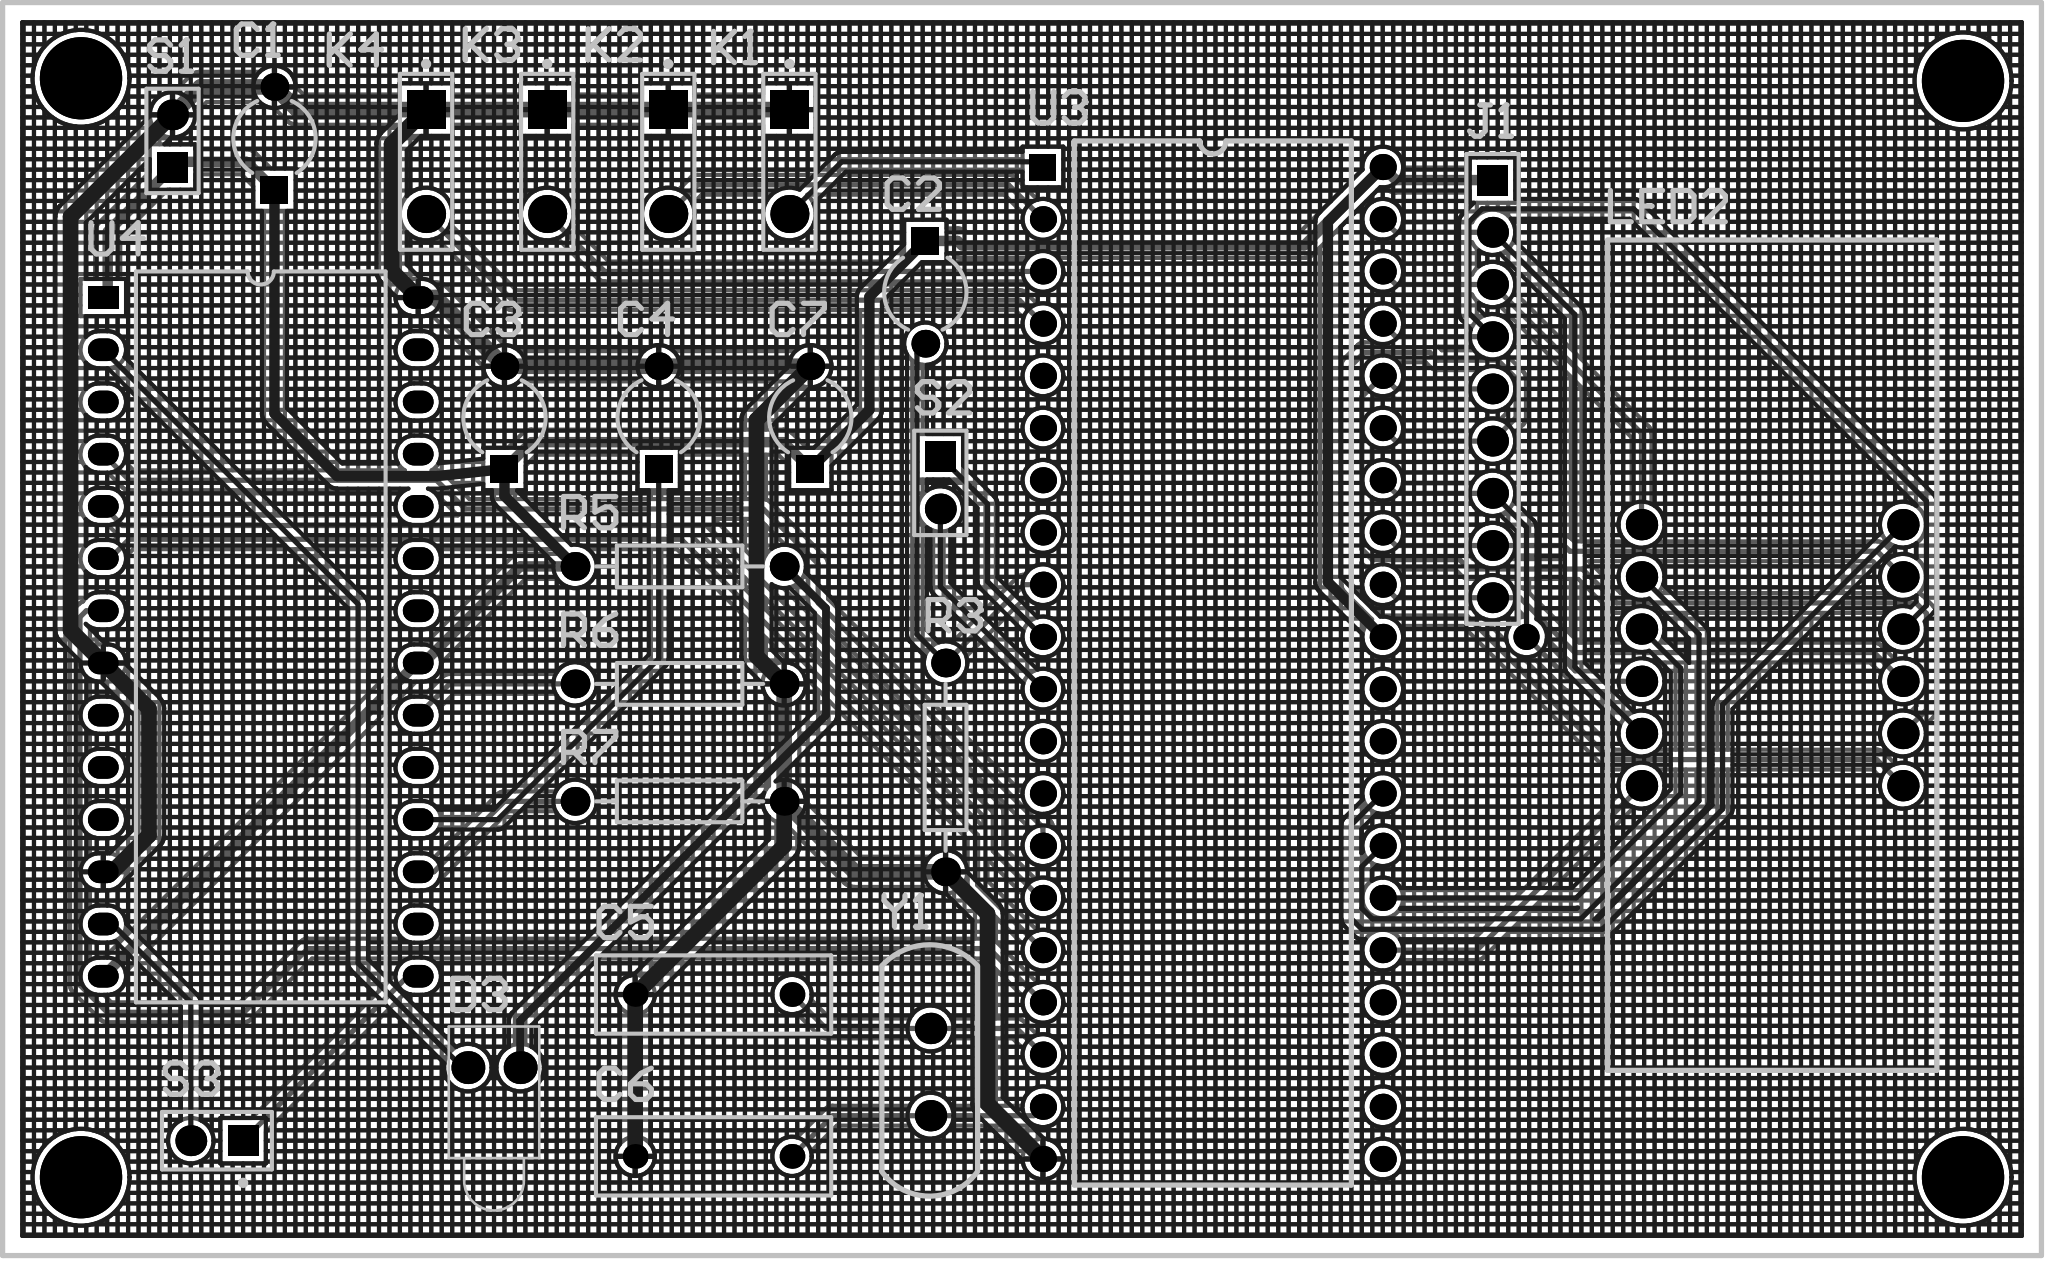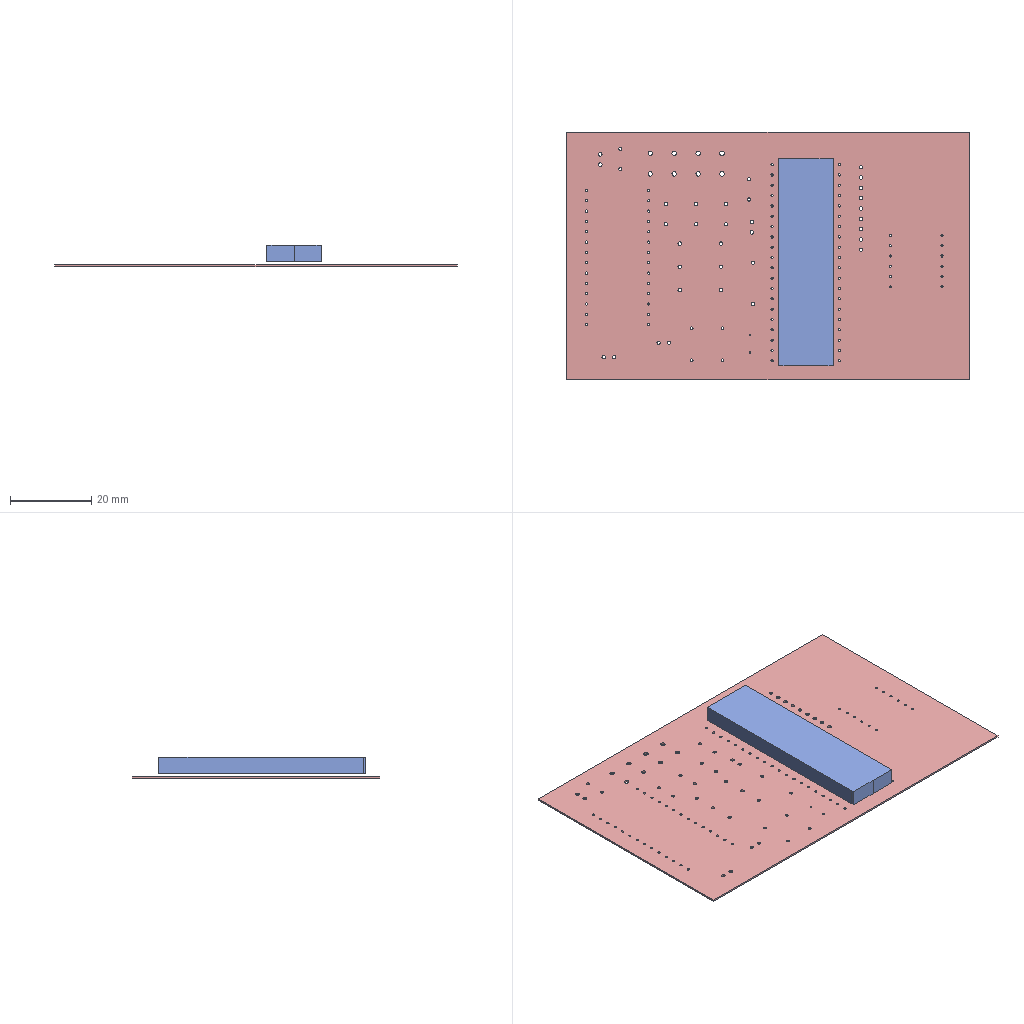Circuit board layout | Altium Designer | box 99.1 x 61 x 5.2 mm
Layer stack:
# Altium Designer layer stack of  (unit mm; dielectric type: 0 none, 1 core, 2 prepreg, 3 surface material)
index,name,kind,layer,copper_thickness_mm,dielectric_type,dielectric_thickness_mm,dielectric_material,dielectric_constant
0,Top Paste,other,,,,,,
1,Top Overlay,other,,,,,,
2,Top Solder,dielectric,,,3,0.0102,Solder Resist,3.5
3,Top Layer,copper,Top Layer,0.0356,,,,
4,Dielectric 1,dielectric,,,0,0.32,FR-4,4.8
5,Bottom Layer,copper,Bottom Layer,0.0356,,,,
6,Bottom Solder,dielectric,,,3,0.0102,Solder Resist,3.5
7,Bottom Overlay,other,,,,,,
8,Bottom Paste,other,,,,,,
# drill layer pairs: low layer,high layer
drill_pair,Top Layer,Bottom Layer
Part placement:
Designator,Comment,Layer,Footprint,Center-X(mm),Center-Y(mm),Rotation
U3,89c51,TopLayer,89c51,104.521,66.929,0
Y1,Component_1,TopLayer,XTAL,90.805,47.026,180
U4,Component_1,TopLayer,ISD1730,58.263,68.199,0
S3,Speaker,TopLayer,PIN2,56.134,43.688,180
S2,Header 2,TopLayer,HDR1X2,91.281,75.692,270
S1,Header 2,TopLayer,HDR1X2,53.975,92.329,90
R7,Res2,TopLayer,AXIAL-0.4,78.613,60.198,180
R6,Res2,TopLayer,AXIAL-0.4,78.613,65.913,180
R5,Res2,TopLayer,AXIAL-0.4,78.613,71.628,360
R3,Res2,TopLayer,AXIAL-0.4,91.535,61.849,90
LED2,Dpy Red-CA,TopLayer,四位数码管,131.699,67.31,90
K4,SW-PB,TopLayer,SPST-2,66.294,91.313,270
K3,SW-PB,TopLayer,SPST-2,72.178,91.313,270
K2,SW-PB,TopLayer,SPST-2,78.063,91.313,270
K1,SW-PB,TopLayer,SPST-2,83.947,91.313,270
J1,Header 9,TopLayer,HDR1X9,118.11,80.264,270
D3,LED1,TopLayer,LED-1,69.596,47.244,270
C7,Cap2,TopLayer,CAPR5-4X5,84.963,78.867,90
C6,Cap,TopLayer,RAD-0.3,80.264,42.926,360
C5,Cap,TopLayer,RAD-0.3,80.264,50.8,360
C4,Cap2,TopLayer,CAPR5-4X5,77.597,78.867,90
C3,Cap2,TopLayer,CAPR5-4X5,70.104,78.867,90
C2,Cap2,TopLayer,CAPR5-4X5,90.551,84.963,270
C1,Cap2,TopLayer,CAPR5-4X5,58.928,92.456,90
Pad and via stacks:
# Altium Designer via and pad stacks of  (unit mm). Each distinct definition once, with the count of objects using it.
# via: kind,start_layer,end_layer,hole_mm,diameter_mm,mode(0 simple;1 top-mid-bottom;2 full stack),diameter_per_layer,count,example_net
# pad: kind,layer,hole_mm,hole_type(0 round;1 square;2 slot),plating,top_size,top_shape(1 round;2 rect;3 octagon;9 rounded rect),mid_size,bottom_size,mode,footprint,size_per_layer,count,example
pad,Multi-Layer,1.1,0,plated,1.85x1.85,2,1.85x1.85,1.85x1.85,0,SPST-2,,4,K1.1
pad,Multi-Layer,1.1,0,plated,1.85x1.85,1,1.85x1.85,1.85x1.85,0,SPST-2,,4,K1.2
pad,Multi-Layer,0.5588,0,plated,1.27x1.27,1,1.27x1.27,1.27x1.27,0,89c51,,39,U3.21
pad,Multi-Layer,0.5588,0,plated,1.27x1.27,2,1.27x1.27,1.27x1.27,0,89c51,,1,U3.1
pad,Multi-Layer,0.51,0,plated,1.524x1.524,1,1.524x1.524,1.524x1.524,0,\u00CB\u00C4\u00CE\u00BB\u00CA\u00FD\u00C2\u00EB\u00B9\u00DC,,12,LED2.1
pad,Multi-Layer,0.9,0,plated,1.5x1.5,2,1.5x1.5,1.5x1.5,0,HDR1X2,,2,S1.1
pad,Multi-Layer,0.9,0,plated,1.5x1.5,1,1.5x1.5,1.5x1.5,0,HDR1X2,,2,S1.2
pad,Multi-Layer,0.8,0,plated,1.35x1.35,1,1.35x1.35,1.35x1.35,0,CAPR5-4X5,,5,C1.2
pad,Multi-Layer,0.8,0,plated,1.35x1.35,2,1.35x1.35,1.35x1.35,0,CAPR5-4X5,,5,C1.1
pad,Multi-Layer,0.9,0,plated,1.5x1.5,2,1.5x1.5,1.5x1.5,0,HDR1X9,,1,J1.1
pad,Multi-Layer,0.9,0,plated,1.5x1.5,1,1.5x1.5,1.5x1.5,0,HDR1X9,,8,J1.3
pad,Multi-Layer,0.85,0,plated,1.4x1.4,1,1.4x1.4,1.4x1.4,0,AXIAL-0.4,,8,R5.1
pad,Multi-Layer,0.8,0,plated,1.6x1.6,1,1.6x1.6,1.6x1.6,0,LED-1,,2,D3.1
pad,Multi-Layer,0.55,0,plated,1.5x1.1,2,1.5x1.1,1.5x1.1,0,ISD1730,,1,U4.1
pad,Multi-Layer,0.55,0,plated,1.5x1.1,1,1.5x1.1,1.5x1.1,0,ISD1730,,27,U4.2
pad,Multi-Layer,0.9,0,plated,1.5x1.5,2,1.5x1.5,1.5x1.5,0,PIN2,,1,S3.1
pad,Multi-Layer,0.9,0,plated,1.5x1.5,1,1.5x1.5,1.5x1.5,0,PIN2,,1,S3.2
pad,Multi-Layer,0.7,0,plated,1.2x1.2,1,1.2x1.2,1.2x1.2,0,RAD-0.3,,4,C5.2
pad,Multi-Layer,0.435,0,plated,1.524x1.524,1,1.524x1.524,1.524x1.524,0,XTAL,,2,Y1.2
via,Top Layer,Bottom Layer,0.7112,1.27,0,,1,P05
via,Top Layer,Bottom Layer,3,4,0,,4,
Copper pours:
name,layer,net,type(0 solid;1 hatched;2 none)
Top Layer-No Net,Top Layer,GND,0
Top Layer-No Net,Bottom Layer,GND,0
Design rules, without the lines most boards share:
# Altium Designer design rules of  (exported by Altium Designer, unit mm)
# columns: name | kind | enabled | priority | scope1 | scope2 | descriptor | typed fields (field=value)
GND | 2 | enabled | 1 | InNet('GND') | All | Width Constraint (Min=10mil) (Max=35mil) (Preferred=30mil) (InNet('GND')) |
VCC | 2 | enabled | 2 | InNet('VCC') | All | Width Constraint (Min=10mil) (Max=25mil) (Preferred=20mil) (InNet('VCC')) |
SilkToSolderMaskClearance | 54 | enabled | 1 | IsPad | All | Silk To Solder Mask (Clearance=0mil) (IsPad),(All) |
MinimumSolderMaskSliver | 53 | enabled | 1 | All | All | Minimum Solder Mask Sliver (Gap=5mil) (All),(All) |
HoleToHoleClearance | 52 | enabled | 1 | All | All | Hole To Hole Clearance (Gap=10mil) (All),(All) | gap=0.254
DiffPairsRouting | 51 | enabled | 1 | All | All | Differential Pairs Uncoupled Length using the Gap Constraints (Min=10mil) (Max=10mil) (Prefered=10mil)  and Width Constraints (Min=15mil) (Max=15mil) (Prefered=15mil) (All) |
HoleSize | 42 | enabled | 1 | All | All | Hole Size Constraint (Min=1mil) (Max=500mil) (All) |
SolderMaskExpansion | 13 | enabled | 1 | All | All | Solder Mask Expansion (Expansion =4mil) (All) | expansion=0.1016
PasteMaskExpansion | 14 | enabled | 1 | All | All | Paste Mask Expansion (Expansion =0mil) (All) | expansion=0
RoutingVias | 11 | enabled | 1 | All | All | Routing Via (MinHoleWidth=28mil) (MaxHoleWidth=28mil) (PreferredHoleWidth=28mil) (MinWidth=50mil) (MaxWidth=50mil) (PreferedWidth=50mil) (All) | via_min_hole=0.7112 via_max_hole=0.7112 via_preferred_diameter=1.27 via_preferred_hole=0.7112
Width | 2 | enabled | 3 | All | All | Width Constraint (Min=8mil) (Max=15mil) (Preferred=10mil) (All) |
PolygonConnect | 20 | enabled | 1 | All | All | Polygon Connect Rule(Relief Connect )(Conductor Width=10mil) (Relief Angle=90 Angle) (Entries=4) (Air Gap Width=10mil) (All),(All) | connect_style(0=relief,1=direct,2=none)=0 relief_conductor_width=0.254 relief_entries=4
PlaneConnect | 6 | enabled | 1 | All | All | Power Plane Connect Rule(Relief Connect )(Expansion=20mil) (Conductor Width=10mil) (Air Gap=10mil) (Entries=4) (All) | relief_conductor_width=0.254 relief_entries=4 relief_expansion=0.508
Clearance | 0 | enabled | 1 | All | All | Clearance Constraint (Gap=10mil) (All),(All) | gap=0.254